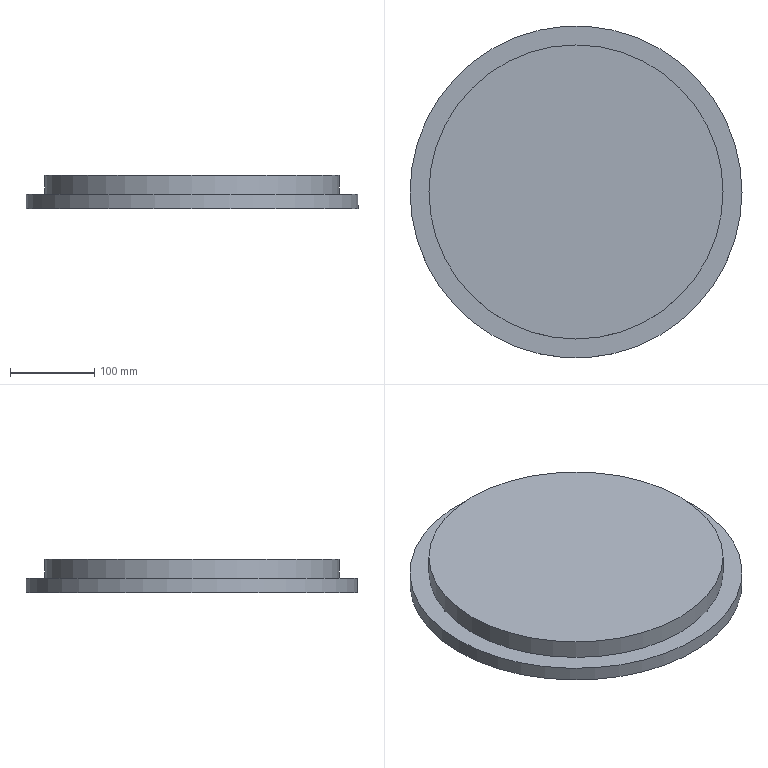Part | NX | features CYLINDER 3, DATUM_CSYS 1, Delete Body 1, LINKED_BODY 1, SCALE 1 | 1 solid | 7 faces | box 393.75 x 393.75 x 39.375 mm | volume 3155764 mm3 | plane 4 | cylinder 3 | commonest cylinder face diameters 281.25 x1 348.75 x1 393.75 x1
STEP:
#1=CARTESIAN_POINT('',(192.207,-1724.979,195.25));
#2=VERTEX_POINT('',#1);
#3=CARTESIAN_POINT('',(366.582,-1724.979,195.25));
#4=DIRECTION('',(0.,0.,-1.));
#5=DIRECTION('',(-1.,0.,0.));
#6=AXIS2_PLACEMENT_3D('',#3,#4,#5);
#7=CIRCLE('',#6,174.375);
#8=EDGE_CURVE('',#2,#2,#7,.T.);
#9=ORIENTED_EDGE('',*,*,#8,.F.);
#10=EDGE_LOOP('',(#9));
#11=FACE_BOUND('',#10,.T.);
#12=CARTESIAN_POINT('',(366.582,-1724.979,195.25));
#13=DIRECTION('',(0.,0.,1.));
#14=DIRECTION('',(1.,0.,0.));
#15=AXIS2_PLACEMENT_3D('',#12,#13,#14);
#16=PLANE('',#15);
#17=ADVANCED_FACE('',(#11),#16,.T.);
#18=CARTESIAN_POINT('',(540.957,-1724.979,172.75));
#19=VERTEX_POINT('',#18);
#20=CARTESIAN_POINT('',(366.582,-1724.979,172.75));
#21=DIRECTION('',(0.,0.,1.));
#22=DIRECTION('',(1.,0.,0.));
#23=AXIS2_PLACEMENT_3D('',#20,#21,#22);
#24=CIRCLE('',#23,174.375);
#25=EDGE_CURVE('',#19,#19,#24,.F.);
#26=ORIENTED_EDGE('',*,*,#25,.F.);
#27=EDGE_LOOP('',(#26));
#28=FACE_BOUND('',#27,.T.);
#29=ORIENTED_EDGE('',*,*,#8,.T.);
#30=EDGE_LOOP('',(#29));
#31=FACE_BOUND('',#30,.T.);
#32=CARTESIAN_POINT('',(366.582,-1724.979,155.875));
#33=DIRECTION('',(0.,0.,1.));
#34=DIRECTION('',(1.,0.,0.));
#35=AXIS2_PLACEMENT_3D('',#32,#33,#34);
#36=CYLINDRICAL_SURFACE('',#35,174.375);
#37=ADVANCED_FACE('',(#28,#31),#36,.T.);
#38=ORIENTED_EDGE('',*,*,#25,.T.);
#39=EDGE_LOOP('',(#38));
#40=FACE_BOUND('',#39,.T.);
#41=CARTESIAN_POINT('',(169.707,-1724.979,172.75));
#42=VERTEX_POINT('',#41);
#43=CARTESIAN_POINT('',(366.582,-1724.979,172.75));
#44=DIRECTION('',(0.,0.,-1.));
#45=DIRECTION('',(-1.,0.,0.));
#46=AXIS2_PLACEMENT_3D('',#43,#44,#45);
#47=CIRCLE('',#46,196.875);
#48=EDGE_CURVE('',#42,#42,#47,.T.);
#49=ORIENTED_EDGE('',*,*,#48,.F.);
#50=EDGE_LOOP('',(#49));
#51=FACE_BOUND('',#50,.T.);
#52=CARTESIAN_POINT('',(366.582,-1724.979,172.75));
#53=DIRECTION('',(0.,0.,1.));
#54=DIRECTION('',(1.,0.,0.));
#55=AXIS2_PLACEMENT_3D('',#52,#53,#54);
#56=PLANE('',#55);
#57=ADVANCED_FACE('',(#40,#51),#56,.T.);
#58=ORIENTED_EDGE('',*,*,#48,.T.);
#59=EDGE_LOOP('',(#58));
#60=FACE_BOUND('',#59,.T.);
#61=CARTESIAN_POINT('',(563.457,-1724.979,155.875));
#62=VERTEX_POINT('',#61);
#63=CARTESIAN_POINT('',(366.582,-1724.979,155.875));
#64=DIRECTION('',(0.,0.,1.));
#65=DIRECTION('',(1.,0.,0.));
#66=AXIS2_PLACEMENT_3D('',#63,#64,#65);
#67=CIRCLE('',#66,196.875);
#68=EDGE_CURVE('',#62,#62,#67,.T.);
#69=ORIENTED_EDGE('',*,*,#68,.T.);
#70=EDGE_LOOP('',(#69));
#71=FACE_BOUND('',#70,.T.);
#72=CARTESIAN_POINT('',(366.582,-1724.979,155.875));
#73=DIRECTION('',(0.,0.,1.));
#74=DIRECTION('',(1.,0.,0.));
#75=AXIS2_PLACEMENT_3D('',#72,#73,#74);
#76=CYLINDRICAL_SURFACE('',#75,196.875);
#77=ADVANCED_FACE('',(#60,#71),#76,.T.);
#78=CARTESIAN_POINT('',(507.207,-1724.979,155.875));
#79=VERTEX_POINT('',#78);
#80=CARTESIAN_POINT('',(366.582,-1724.979,155.875));
#81=DIRECTION('',(0.,0.,1.));
#82=DIRECTION('',(1.,0.,0.));
#83=AXIS2_PLACEMENT_3D('',#80,#81,#82);
#84=CIRCLE('',#83,140.625);
#85=EDGE_CURVE('',#79,#79,#84,.T.);
#86=ORIENTED_EDGE('',*,*,#85,.T.);
#87=EDGE_LOOP('',(#86));
#88=FACE_BOUND('',#87,.T.);
#89=ORIENTED_EDGE('',*,*,#68,.F.);
#90=EDGE_LOOP('',(#89));
#91=FACE_BOUND('',#90,.T.);
#92=CARTESIAN_POINT('',(366.582,-1724.979,155.875));
#93=DIRECTION('',(0.,0.,-1.));
#94=DIRECTION('',(-1.,0.,0.));
#95=AXIS2_PLACEMENT_3D('',#92,#93,#94);
#96=PLANE('',#95);
#97=ADVANCED_FACE('',(#88,#91),#96,.T.);
#98=CARTESIAN_POINT('',(225.957,-1724.979,172.75));
#99=VERTEX_POINT('',#98);
#100=CARTESIAN_POINT('',(366.582,-1724.979,172.75));
#101=DIRECTION('',(0.,0.,-1.));
#102=DIRECTION('',(-1.,0.,0.));
#103=AXIS2_PLACEMENT_3D('',#100,#101,#102);
#104=CIRCLE('',#103,140.625);
#105=EDGE_CURVE('',#99,#99,#104,.F.);
#106=ORIENTED_EDGE('',*,*,#105,.F.);
#107=EDGE_LOOP('',(#106));
#108=FACE_BOUND('',#107,.T.);
#109=CARTESIAN_POINT('',(366.582,-1724.979,172.75));
#110=DIRECTION('',(0.,0.,1.));
#111=DIRECTION('',(1.,0.,0.));
#112=AXIS2_PLACEMENT_3D('',#109,#110,#111);
#113=PLANE('',#112);
#114=ADVANCED_FACE('',(#108),#113,.F.);
#115=ORIENTED_EDGE('',*,*,#105,.T.);
#116=EDGE_LOOP('',(#115));
#117=FACE_BOUND('',#116,.T.);
#118=ORIENTED_EDGE('',*,*,#85,.F.);
#119=EDGE_LOOP('',(#118));
#120=FACE_BOUND('',#119,.T.);
#121=CARTESIAN_POINT('',(366.582,-1724.979,155.875));
#122=DIRECTION('',(0.,0.,1.));
#123=DIRECTION('',(1.,0.,0.));
#124=AXIS2_PLACEMENT_3D('',#121,#122,#123);
#125=CYLINDRICAL_SURFACE('',#124,140.625);
#126=ADVANCED_FACE('',(#117,#120),#125,.F.);
#127=CLOSED_SHELL('',(#17,#37,#57,#77,#97,#114,#126));
#128=MANIFOLD_SOLID_BREP('',#127);
#129=(LENGTH_UNIT()NAMED_UNIT(*)SI_UNIT(.MILLI.,.METRE.));
#130=UNCERTAINTY_MEASURE_WITH_UNIT(LENGTH_MEASURE(0.00001),#129,'','');
#131=(NAMED_UNIT(*)PLANE_ANGLE_UNIT()SI_UNIT($,.RADIAN.));
#132=(NAMED_UNIT(*)SI_UNIT($,.STERADIAN.)SOLID_ANGLE_UNIT());
#133=(GEOMETRIC_REPRESENTATION_CONTEXT(3)GLOBAL_UNCERTAINTY_ASSIGNED_CONTEXT((#130))GLOBAL_UNIT_ASSIGNED_CONTEXT((#129,#131,#132))REPRESENTATION_CONTEXT('',''));
#134=ADVANCED_BREP_SHAPE_REPRESENTATION('',(#128),#133);